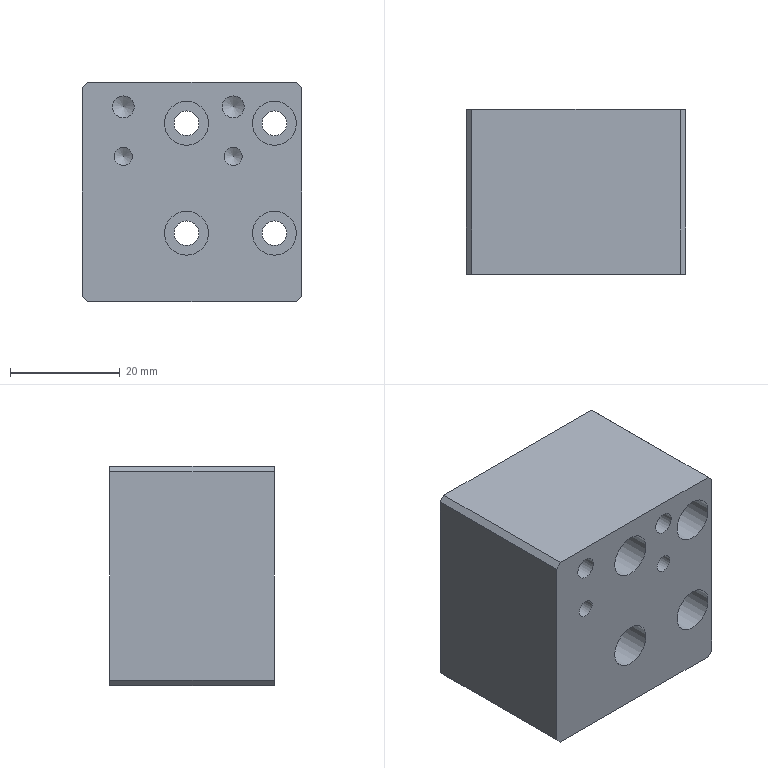CAM job | NX | 3+2 milling, drilling | part box 40 x 30 x 40 mm | stock box 45 x 35 x 45 mm
Tools:
number,name,description,diameter,corner_radius,flute_length,length,flutes
18,D2,平底铣刀-粗,2.0,0.0,50.0,75.0,2
4,D4,平底铣刀-粗,4.0,0.0,25.0,75.0,2
9,D10,平底铣刀-粗,10.0,0.0,35.0,75.0,2
19,D2-J,平底铣刀-精,2.0,0.0,50.0,75.0,2
17,D4-J,平底铣刀-精,4.0,0.0,50.0,75.0,2
10,D10-J,平底铣刀-精,10.0,0.0,35.0,75.0,2
1,D80R0.8_FLYCUTTER,圆鼻刀-粗,80.0,0.8,50.0,75.0,2
2,D6_CHAMFERCUTTER,倒角刀,6.0,0.0,3.0,25.0,2
21,M4X0.7,丝锥,3.3,0.0,35.0,50.0,2
13,ZT3.3,钻头,3.3,0.0,35.0,50.0,2
11,ZT4.5,钻头,4.5,0.0,35.0,50.0,2
13,DRILL3.3,Twist Drill 3.3 mm,3.3,0.0,35.0,35.008,2
Operations:
program,operation,operation_type,tool,method,geometry_group,spindle_rpm,surface_speed,feed_per_tooth,feed_cut,feed_plunge,cut_length_mm,path_length_mm,cut_time_min,machine_time_min
A,TOP_FACE,FaceMilling,D80R0.8_FLYCUTTER,SIDEMILL_FINISH-DEPTHK-STEPG,W-A,5000.0,1256.637,0.1,1000.0,100.0,134.0,170.0,0.134,0.1376
A,PROFILE_ROUGH_2,VolumeBased25DMillingOperation,D10,METHOD,W-A,8000.0,251.327,0.3125,5000.0,80.0,7589.608,7658.408,1.518,1.525
A,SPOTDRILL-DEPTH0.8,Operation,D6_CHAMFERCUTTER,NONE,W-A,8000.0,150.796,0.0312,500.0,90.0,14.4,155.593,0.0288,0.0429
A,COUNTERBORE-DRILL_SEG0,Operation,ZT4.5,NONE,W-A,2800.0,39.584,0.0536,300.0,90.0,137.408,369.903,0.458,0.4813
A,BLINDTAPER-M4_TAPDRILL,Operation,DRILL3.3,NONE,W-A,3000.0,31.102,0.0333,200.0,90.0,24.183,109.391,0.1209,0.1294
A,BLINDTAPER-REAM4.0_PREDRILL,Operation,ZT3.3,NONE,W-A,3000.0,35.814,0.0333,200.0,90.0,24.403,109.832,0.122,0.1306
A,HOLEMILL_ROUGH_D4_1,CylinderMilling,D4,NONE,W-A,8000.0,100.531,0.075,1200.0,100.0,4131.847,4441.847,3.443,3.474
A,HOLEMILL_FINISH_D4_1,CylinderMilling,D4-J,FINISH_STEPDEPTHOFF,W-A,8000.0,100.531,0.0312,500.0,100.0,351.069,661.069,0.7021,0.7331
A,HOLEMILL_ROUGH_D2_1,CylinderMilling,D2,NONE,W-A,8000.0,50.266,0.0375,600.0,100.0,435.628,554.828,0.726,0.738
A,SELECTBODYONLY,SurfaceContour,D6_CHAMFERCUTTER,METHOD,W-A,8000.0,150.796,0.1875,3000.0,100.0,174.958,210.76,0.0583,0.0619
A,DRILLCHAMFER_1,Operation,D6_CHAMFERCUTTER,METHOD,W-A,8000.0,150.796,0.0312,500.0,0.0,10.4,84.024,0.0208,0.0282
A,DRILLCHAMFER_2,Operation,D6_CHAMFERCUTTER,METHOD,W-A,8000.0,150.796,0.0312,500.0,0.0,10.6,84.424,0.0212,0.0286
A,MILLCHAMFER_1,PlanarMilling,D6_CHAMFERCUTTER,NONE,W-A,8000.0,150.796,0.0312,500.0,100.0,135.871,327.988,0.2717,0.291
A,BLINDTAPER-TAPM4,Operation,M4X0.7,METHOD,W-A,800.0,8.294,0.0004,0.7,90.0,18.2,97.425,26.0,26.008
A,HOLEMILL_FINISH_D2_1,CylinderMilling,D2-J,FINISH_STEPDEPTHOFF,W-A,8000.0,50.266,0.0125,200.0,100.0,293.005,412.204,1.465,1.477
A,PROFILE_SEMIFINISH_2,VolumeBased25DMillingOperation,D10-J,METHOD,W-A,8000.0,251.327,0.0625,1000.0,100.0,388.062,559.476,0.3881,0.4052